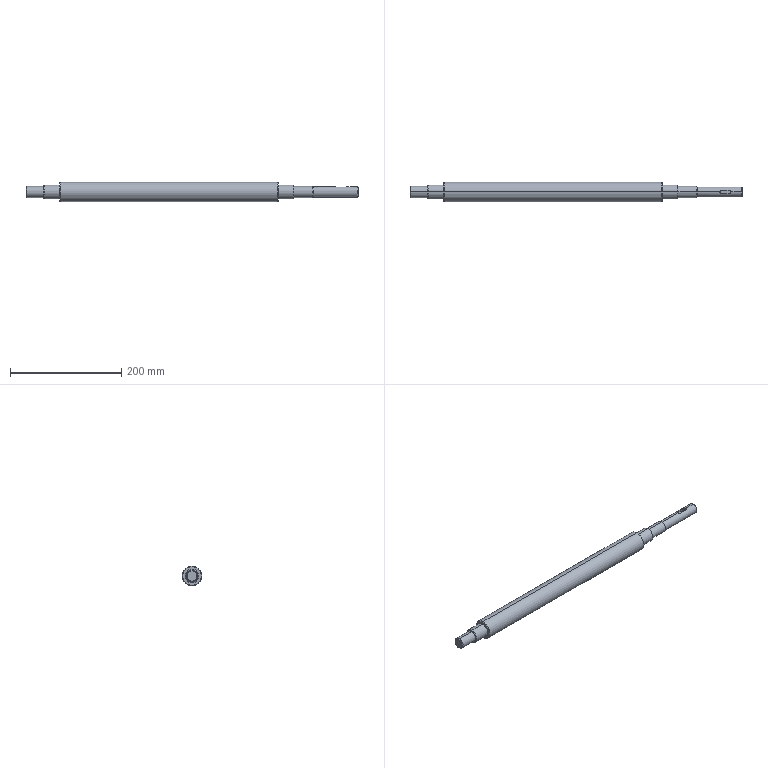Part | STEP file | Flat conveyor mechanism-CN2500x400-107-101 | 1 solid | 49 faces | box 595.6 x 35 x 35 mm | volume 445688 mm3 | cylinder 20 | cone 14 | plane 11 | torus 4 | commonest cylinder face diameters 0.4 x4 6 x4 20 x4 25 x4 18 x2 35 x2
STEP:
#1=CARTESIAN_POINT('',(-256.4,0.,9.));
#2=VERTEX_POINT('',#1);
#3=CARTESIAN_POINT('',(-256.4,0.,-9.));
#4=VERTEX_POINT('',#3);
#5=CARTESIAN_POINT('',(-256.4,0.,0.));
#6=DIRECTION('',(-1.,0.,0.));
#7=DIRECTION('',(0.,0.,-1.));
#8=AXIS2_PLACEMENT_3D('',#5,#6,#7);
#9=CIRCLE('',#8,9.);
#10=EDGE_CURVE('',#2,#4,#9,.T.);
#11=ORIENTED_EDGE('',*,*,#10,.F.);
#12=CARTESIAN_POINT('',(-255.4,0.,10.));
#13=VERTEX_POINT('',#12);
#14=CARTESIAN_POINT('',(-256.4,0.,9.));
#15=DIRECTION('',(0.7071,0.,0.7071));
#16=VECTOR('',#15,1000.);
#17=LINE('',#14,#16);
#18=EDGE_CURVE('',#2,#13,#17,.T.);
#19=ORIENTED_EDGE('',*,*,#18,.T.);
#20=CARTESIAN_POINT('',(-255.4,0.,-10.));
#21=VERTEX_POINT('',#20);
#22=CARTESIAN_POINT('',(-255.4,0.,0.));
#23=DIRECTION('',(1.,0.,0.));
#24=DIRECTION('',(0.,0.,-1.));
#25=AXIS2_PLACEMENT_3D('',#22,#23,#24);
#26=CIRCLE('',#25,10.);
#27=EDGE_CURVE('',#21,#13,#26,.T.);
#28=ORIENTED_EDGE('',*,*,#27,.F.);
#29=CARTESIAN_POINT('',(-256.4,0.,-9.));
#30=DIRECTION('',(0.7071,0.,-0.7071));
#31=VECTOR('',#30,1000.);
#32=LINE('',#29,#31);
#33=EDGE_CURVE('',#4,#21,#32,.T.);
#34=ORIENTED_EDGE('',*,*,#33,.F.);
#35=EDGE_LOOP('',(#11,#19,#28,#34));
#36=FACE_OUTER_BOUND('',#35,.T.);
#37=CARTESIAN_POINT('',(-256.4,0.,0.));
#38=DIRECTION('',(1.,0.,0.));
#39=DIRECTION('',(0.,0.,-1.));
#40=AXIS2_PLACEMENT_3D('',#37,#38,#39);
#41=CONICAL_SURFACE('',#40,9.,0.7854);
#42=ADVANCED_FACE('',(#36),#41,.T.);
#43=CARTESIAN_POINT('',(-224.4,0.,11.5));
#44=VERTEX_POINT('',#43);
#45=CARTESIAN_POINT('',(-224.4,0.,-11.5));
#46=VERTEX_POINT('',#45);
#47=CARTESIAN_POINT('',(-224.4,0.,0.));
#48=DIRECTION('',(-1.,0.,0.));
#49=DIRECTION('',(0.,0.,-1.));
#50=AXIS2_PLACEMENT_3D('',#47,#48,#49);
#51=CIRCLE('',#50,11.5);
#52=EDGE_CURVE('',#44,#46,#51,.T.);
#53=ORIENTED_EDGE('',*,*,#52,.F.);
#54=CARTESIAN_POINT('',(-223.4,0.,12.5));
#55=VERTEX_POINT('',#54);
#56=CARTESIAN_POINT('',(-224.4,0.,11.5));
#57=DIRECTION('',(0.7071,0.,0.7071));
#58=VECTOR('',#57,1000.);
#59=LINE('',#56,#58);
#60=EDGE_CURVE('',#44,#55,#59,.T.);
#61=ORIENTED_EDGE('',*,*,#60,.T.);
#62=CARTESIAN_POINT('',(-223.4,0.,-12.5));
#63=VERTEX_POINT('',#62);
#64=CARTESIAN_POINT('',(-223.4,0.,0.));
#65=DIRECTION('',(1.,0.,0.));
#66=DIRECTION('',(0.,0.,-1.));
#67=AXIS2_PLACEMENT_3D('',#64,#65,#66);
#68=CIRCLE('',#67,12.5);
#69=EDGE_CURVE('',#63,#55,#68,.T.);
#70=ORIENTED_EDGE('',*,*,#69,.F.);
#71=CARTESIAN_POINT('',(-224.4,0.,-11.5));
#72=DIRECTION('',(0.7071,0.,-0.7071));
#73=VECTOR('',#72,1000.);
#74=LINE('',#71,#73);
#75=EDGE_CURVE('',#46,#63,#74,.T.);
#76=ORIENTED_EDGE('',*,*,#75,.F.);
#77=EDGE_LOOP('',(#53,#61,#70,#76));
#78=FACE_OUTER_BOUND('',#77,.T.);
#79=CARTESIAN_POINT('',(-224.4,0.,0.));
#80=DIRECTION('',(1.,0.,0.));
#81=DIRECTION('',(0.,0.,-1.));
#82=AXIS2_PLACEMENT_3D('',#79,#80,#81);
#83=CONICAL_SURFACE('',#82,11.5,0.7854);
#84=ADVANCED_FACE('',(#78),#83,.T.);
#85=CARTESIAN_POINT('',(-196.1,0.,16.5));
#86=VERTEX_POINT('',#85);
#87=CARTESIAN_POINT('',(-196.1,0.,-16.5));
#88=VERTEX_POINT('',#87);
#89=CARTESIAN_POINT('',(-196.1,0.,0.));
#90=DIRECTION('',(-1.,0.,0.));
#91=DIRECTION('',(0.,0.,-1.));
#92=AXIS2_PLACEMENT_3D('',#89,#90,#91);
#93=CIRCLE('',#92,16.5);
#94=EDGE_CURVE('',#86,#88,#93,.T.);
#95=ORIENTED_EDGE('',*,*,#94,.F.);
#96=CARTESIAN_POINT('',(-195.1,0.,17.5));
#97=VERTEX_POINT('',#96);
#98=CARTESIAN_POINT('',(-196.1,0.,16.5));
#99=DIRECTION('',(0.7071,0.,0.7071));
#100=VECTOR('',#99,1000.);
#101=LINE('',#98,#100);
#102=EDGE_CURVE('',#86,#97,#101,.T.);
#103=ORIENTED_EDGE('',*,*,#102,.T.);
#104=CARTESIAN_POINT('',(-195.1,0.,-17.5));
#105=VERTEX_POINT('',#104);
#106=CARTESIAN_POINT('',(-195.1,0.,0.));
#107=DIRECTION('',(1.,0.,0.));
#108=DIRECTION('',(0.,0.,-1.));
#109=AXIS2_PLACEMENT_3D('',#106,#107,#108);
#110=CIRCLE('',#109,17.5);
#111=EDGE_CURVE('',#105,#97,#110,.T.);
#112=ORIENTED_EDGE('',*,*,#111,.F.);
#113=CARTESIAN_POINT('',(-196.1,0.,-16.5));
#114=DIRECTION('',(0.7071,0.,-0.7071));
#115=VECTOR('',#114,1000.);
#116=LINE('',#113,#115);
#117=EDGE_CURVE('',#88,#105,#116,.T.);
#118=ORIENTED_EDGE('',*,*,#117,.F.);
#119=EDGE_LOOP('',(#95,#103,#112,#118));
#120=FACE_OUTER_BOUND('',#119,.T.);
#121=CARTESIAN_POINT('',(-196.1,0.,0.));
#122=DIRECTION('',(1.,0.,0.));
#123=DIRECTION('',(0.,0.,-1.));
#124=AXIS2_PLACEMENT_3D('',#121,#122,#123);
#125=CONICAL_SURFACE('',#124,16.5,0.7854);
#126=ADVANCED_FACE('',(#120),#125,.T.);
#127=CARTESIAN_POINT('',(195.9,0.,-16.5));
#128=VERTEX_POINT('',#127);
#129=CARTESIAN_POINT('',(195.9,0.,16.5));
#130=VERTEX_POINT('',#129);
#131=CARTESIAN_POINT('',(195.9,0.,0.));
#132=DIRECTION('',(1.,0.,0.));
#133=DIRECTION('',(0.,0.,1.));
#134=AXIS2_PLACEMENT_3D('',#131,#132,#133);
#135=CIRCLE('',#134,16.5);
#136=EDGE_CURVE('',#128,#130,#135,.T.);
#137=ORIENTED_EDGE('',*,*,#136,.F.);
#138=CARTESIAN_POINT('',(194.9,0.,-17.5));
#139=VERTEX_POINT('',#138);
#140=CARTESIAN_POINT('',(194.9,0.,-17.5));
#141=DIRECTION('',(-0.7071,0.,-0.7071));
#142=VECTOR('',#141,1000.);
#143=LINE('',#140,#142);
#144=EDGE_CURVE('',#128,#139,#143,.T.);
#145=ORIENTED_EDGE('',*,*,#144,.T.);
#146=CARTESIAN_POINT('',(194.9,0.,17.5));
#147=VERTEX_POINT('',#146);
#148=CARTESIAN_POINT('',(194.9,0.,0.));
#149=DIRECTION('',(-1.,0.,0.));
#150=DIRECTION('',(0.,0.,1.));
#151=AXIS2_PLACEMENT_3D('',#148,#149,#150);
#152=CIRCLE('',#151,17.5);
#153=EDGE_CURVE('',#147,#139,#152,.T.);
#154=ORIENTED_EDGE('',*,*,#153,.F.);
#155=CARTESIAN_POINT('',(194.9,0.,17.5));
#156=DIRECTION('',(-0.7071,0.,0.7071));
#157=VECTOR('',#156,1000.);
#158=LINE('',#155,#157);
#159=EDGE_CURVE('',#130,#147,#158,.T.);
#160=ORIENTED_EDGE('',*,*,#159,.F.);
#161=EDGE_LOOP('',(#137,#145,#154,#160));
#162=FACE_OUTER_BOUND('',#161,.T.);
#163=CARTESIAN_POINT('',(194.9,0.,0.));
#164=DIRECTION('',(-1.,0.,0.));
#165=DIRECTION('',(0.,0.,1.));
#166=AXIS2_PLACEMENT_3D('',#163,#164,#165);
#167=CONICAL_SURFACE('',#166,17.5,0.7854);
#168=ADVANCED_FACE('',(#162),#167,.T.);
#169=CARTESIAN_POINT('',(224.2,0.,-11.5));
#170=VERTEX_POINT('',#169);
#171=CARTESIAN_POINT('',(224.2,0.,11.5));
#172=VERTEX_POINT('',#171);
#173=CARTESIAN_POINT('',(224.2,0.,0.));
#174=DIRECTION('',(1.,0.,0.));
#175=DIRECTION('',(0.,0.,1.));
#176=AXIS2_PLACEMENT_3D('',#173,#174,#175);
#177=CIRCLE('',#176,11.5);
#178=EDGE_CURVE('',#170,#172,#177,.T.);
#179=ORIENTED_EDGE('',*,*,#178,.F.);
#180=CARTESIAN_POINT('',(223.2,0.,-12.5));
#181=VERTEX_POINT('',#180);
#182=CARTESIAN_POINT('',(223.2,0.,-12.5));
#183=DIRECTION('',(-0.7071,0.,-0.7071));
#184=VECTOR('',#183,1000.);
#185=LINE('',#182,#184);
#186=EDGE_CURVE('',#170,#181,#185,.T.);
#187=ORIENTED_EDGE('',*,*,#186,.T.);
#188=CARTESIAN_POINT('',(223.2,0.,12.5));
#189=VERTEX_POINT('',#188);
#190=CARTESIAN_POINT('',(223.2,0.,0.));
#191=DIRECTION('',(-1.,0.,0.));
#192=DIRECTION('',(0.,0.,1.));
#193=AXIS2_PLACEMENT_3D('',#190,#191,#192);
#194=CIRCLE('',#193,12.5);
#195=EDGE_CURVE('',#189,#181,#194,.T.);
#196=ORIENTED_EDGE('',*,*,#195,.F.);
#197=CARTESIAN_POINT('',(223.2,0.,12.5));
#198=DIRECTION('',(-0.7071,0.,0.7071));
#199=VECTOR('',#198,1000.);
#200=LINE('',#197,#199);
#201=EDGE_CURVE('',#172,#189,#200,.T.);
#202=ORIENTED_EDGE('',*,*,#201,.F.);
#203=EDGE_LOOP('',(#179,#187,#196,#202));
#204=FACE_OUTER_BOUND('',#203,.T.);
#205=CARTESIAN_POINT('',(223.2,0.,0.));
#206=DIRECTION('',(-1.,0.,0.));
#207=DIRECTION('',(0.,0.,1.));
#208=AXIS2_PLACEMENT_3D('',#205,#206,#207);
#209=CONICAL_SURFACE('',#208,12.5,0.7854);
#210=ADVANCED_FACE('',(#204),#209,.T.);
#211=CARTESIAN_POINT('',(259.2,0.,9.));
#212=VERTEX_POINT('',#211);
#213=CARTESIAN_POINT('',(259.2,0.,-9.));
#214=VERTEX_POINT('',#213);
#215=CARTESIAN_POINT('',(259.2,0.,0.));
#216=DIRECTION('',(-1.,0.,0.));
#217=DIRECTION('',(0.,0.,1.));
#218=AXIS2_PLACEMENT_3D('',#215,#216,#217);
#219=CIRCLE('',#218,9.);
#220=EDGE_CURVE('',#212,#214,#219,.T.);
#221=ORIENTED_EDGE('',*,*,#220,.T.);
#222=CARTESIAN_POINT('',(258.2,0.,-10.));
#223=VERTEX_POINT('',#222);
#224=CARTESIAN_POINT('',(258.2,0.,-10.));
#225=DIRECTION('',(-0.7071,0.,-0.7071));
#226=VECTOR('',#225,1000.);
#227=LINE('',#224,#226);
#228=EDGE_CURVE('',#214,#223,#227,.T.);
#229=ORIENTED_EDGE('',*,*,#228,.T.);
#230=CARTESIAN_POINT('',(258.2,0.,10.));
#231=VERTEX_POINT('',#230);
#232=CARTESIAN_POINT('',(258.2,0.,0.));
#233=DIRECTION('',(-1.,0.,0.));
#234=DIRECTION('',(0.,0.,1.));
#235=AXIS2_PLACEMENT_3D('',#232,#233,#234);
#236=CIRCLE('',#235,10.);
#237=EDGE_CURVE('',#231,#223,#236,.T.);
#238=ORIENTED_EDGE('',*,*,#237,.F.);
#239=CARTESIAN_POINT('',(258.2,0.,10.));
#240=DIRECTION('',(-0.7071,0.,0.7071));
#241=VECTOR('',#240,1000.);
#242=LINE('',#239,#241);
#243=EDGE_CURVE('',#212,#231,#242,.T.);
#244=ORIENTED_EDGE('',*,*,#243,.F.);
#245=EDGE_LOOP('',(#221,#229,#238,#244));
#246=FACE_OUTER_BOUND('',#245,.T.);
#247=CARTESIAN_POINT('',(258.2,0.,0.));
#248=DIRECTION('',(-1.,0.,0.));
#249=DIRECTION('',(0.,0.,1.));
#250=AXIS2_PLACEMENT_3D('',#247,#248,#249);
#251=CONICAL_SURFACE('',#250,10.,0.7854);
#252=ADVANCED_FACE('',(#246),#251,.T.);
#253=CARTESIAN_POINT('',(339.2,0.,-8.));
#254=VERTEX_POINT('',#253);
#255=CARTESIAN_POINT('',(339.2,0.,8.));
#256=VERTEX_POINT('',#255);
#257=CARTESIAN_POINT('',(339.2,0.,0.));
#258=DIRECTION('',(1.,0.,0.));
#259=DIRECTION('',(0.,0.,1.));
#260=AXIS2_PLACEMENT_3D('',#257,#258,#259);
#261=CIRCLE('',#260,8.);
#262=EDGE_CURVE('',#254,#256,#261,.T.);
#263=ORIENTED_EDGE('',*,*,#262,.F.);
#264=CARTESIAN_POINT('',(338.2,0.,-9.));
#265=VERTEX_POINT('',#264);
#266=CARTESIAN_POINT('',(338.2,0.,-9.));
#267=DIRECTION('',(-0.7071,0.,-0.7071));
#268=VECTOR('',#267,1000.);
#269=LINE('',#266,#268);
#270=EDGE_CURVE('',#254,#265,#269,.T.);
#271=ORIENTED_EDGE('',*,*,#270,.T.);
#272=CARTESIAN_POINT('',(338.2,0.,9.));
#273=VERTEX_POINT('',#272);
#274=CARTESIAN_POINT('',(338.2,0.,0.));
#275=DIRECTION('',(-1.,0.,0.));
#276=DIRECTION('',(0.,0.,1.));
#277=AXIS2_PLACEMENT_3D('',#274,#275,#276);
#278=CIRCLE('',#277,9.);
#279=EDGE_CURVE('',#273,#265,#278,.T.);
#280=ORIENTED_EDGE('',*,*,#279,.F.);
#281=CARTESIAN_POINT('',(338.2,0.,9.));
#282=DIRECTION('',(-0.7071,0.,0.7071));
#283=VECTOR('',#282,1000.);
#284=LINE('',#281,#283);
#285=EDGE_CURVE('',#256,#273,#284,.T.);
#286=ORIENTED_EDGE('',*,*,#285,.F.);
#287=EDGE_LOOP('',(#263,#271,#280,#286));
#288=FACE_OUTER_BOUND('',#287,.T.);
#289=CARTESIAN_POINT('',(338.2,0.,0.));
#290=DIRECTION('',(-1.,0.,0.));
#291=DIRECTION('',(0.,0.,1.));
#292=AXIS2_PLACEMENT_3D('',#289,#290,#291);
#293=CONICAL_SURFACE('',#292,9.,0.7854);
#294=ADVANCED_FACE('',(#288),#293,.T.);
#295=CARTESIAN_POINT('',(-224.4,0.,10.));
#296=VERTEX_POINT('',#295);
#297=CARTESIAN_POINT('',(-224.4,0.,-10.));
#298=VERTEX_POINT('',#297);
#299=CARTESIAN_POINT('',(-224.4,0.,0.));
#300=DIRECTION('',(-1.,0.,0.));
#301=DIRECTION('',(0.,0.,1.));
#302=AXIS2_PLACEMENT_3D('',#299,#300,#301);
#303=CIRCLE('',#302,10.);
#304=EDGE_CURVE('',#296,#298,#303,.T.);
#305=ORIENTED_EDGE('',*,*,#304,.T.);
#306=CARTESIAN_POINT('',(-209.5,0.,-10.));
#307=DIRECTION('',(-1.,0.,0.));
#308=VECTOR('',#307,1000.);
#309=LINE('',#306,#308);
#310=EDGE_CURVE('',#298,#21,#309,.T.);
#311=ORIENTED_EDGE('',*,*,#310,.T.);
#312=ORIENTED_EDGE('',*,*,#27,.T.);
#313=CARTESIAN_POINT('',(-209.5,0.,10.));
#314=DIRECTION('',(-1.,0.,0.));
#315=VECTOR('',#314,1000.);
#316=LINE('',#313,#315);
#317=EDGE_CURVE('',#296,#13,#316,.T.);
#318=ORIENTED_EDGE('',*,*,#317,.F.);
#319=EDGE_LOOP('',(#305,#311,#312,#318));
#320=FACE_OUTER_BOUND('',#319,.T.);
#321=CARTESIAN_POINT('',(-209.5,0.,0.));
#322=DIRECTION('',(-1.,0.,0.));
#323=DIRECTION('',(0.,0.,1.));
#324=AXIS2_PLACEMENT_3D('',#321,#322,#323);
#325=CYLINDRICAL_SURFACE('',#324,10.);
#326=ADVANCED_FACE('',(#320),#325,.T.);
#327=CARTESIAN_POINT('',(-196.1,0.,12.5));
#328=VERTEX_POINT('',#327);
#329=CARTESIAN_POINT('',(-196.1,0.,-12.5));
#330=VERTEX_POINT('',#329);
#331=CARTESIAN_POINT('',(-196.1,0.,0.));
#332=DIRECTION('',(-1.,0.,0.));
#333=DIRECTION('',(0.,0.,1.));
#334=AXIS2_PLACEMENT_3D('',#331,#332,#333);
#335=CIRCLE('',#334,12.5);
#336=EDGE_CURVE('',#328,#330,#335,.T.);
#337=ORIENTED_EDGE('',*,*,#336,.T.);
#338=CARTESIAN_POINT('',(-209.5,0.,-12.5));
#339=DIRECTION('',(-1.,0.,0.));
#340=VECTOR('',#339,1000.);
#341=LINE('',#338,#340);
#342=EDGE_CURVE('',#330,#63,#341,.T.);
#343=ORIENTED_EDGE('',*,*,#342,.T.);
#344=ORIENTED_EDGE('',*,*,#69,.T.);
#345=CARTESIAN_POINT('',(-209.5,0.,12.5));
#346=DIRECTION('',(-1.,0.,0.));
#347=VECTOR('',#346,1000.);
#348=LINE('',#345,#347);
#349=EDGE_CURVE('',#328,#55,#348,.T.);
#350=ORIENTED_EDGE('',*,*,#349,.F.);
#351=EDGE_LOOP('',(#337,#343,#344,#350));
#352=FACE_OUTER_BOUND('',#351,.T.);
#353=CARTESIAN_POINT('',(-209.5,0.,0.));
#354=DIRECTION('',(-1.,0.,0.));
#355=DIRECTION('',(0.,0.,1.));
#356=AXIS2_PLACEMENT_3D('',#353,#354,#355);
#357=CYLINDRICAL_SURFACE('',#356,12.5);
#358=ADVANCED_FACE('',(#352),#357,.T.);
#359=ORIENTED_EDGE('',*,*,#153,.T.);
#360=CARTESIAN_POINT('',(-209.5,0.,-17.5));
#361=DIRECTION('',(-1.,0.,0.));
#362=VECTOR('',#361,1000.);
#363=LINE('',#360,#362);
#364=EDGE_CURVE('',#139,#105,#363,.T.);
#365=ORIENTED_EDGE('',*,*,#364,.T.);
#366=ORIENTED_EDGE('',*,*,#111,.T.);
#367=CARTESIAN_POINT('',(-209.5,0.,17.5));
#368=DIRECTION('',(-1.,0.,0.));
#369=VECTOR('',#368,1000.);
#370=LINE('',#367,#369);
#371=EDGE_CURVE('',#147,#97,#370,.T.);
#372=ORIENTED_EDGE('',*,*,#371,.F.);
#373=EDGE_LOOP('',(#359,#365,#366,#372));
#374=FACE_OUTER_BOUND('',#373,.T.);
#375=CARTESIAN_POINT('',(-209.5,0.,0.));
#376=DIRECTION('',(-1.,0.,0.));
#377=DIRECTION('',(0.,0.,1.));
#378=AXIS2_PLACEMENT_3D('',#375,#376,#377);
#379=CYLINDRICAL_SURFACE('',#378,17.5);
#380=ADVANCED_FACE('',(#374),#379,.T.);
#381=ORIENTED_EDGE('',*,*,#195,.T.);
#382=CARTESIAN_POINT('',(195.9,0.,-12.5));
#383=VERTEX_POINT('',#382);
#384=CARTESIAN_POINT('',(-209.5,0.,-12.5));
#385=DIRECTION('',(-1.,0.,0.));
#386=VECTOR('',#385,1000.);
#387=LINE('',#384,#386);
#388=EDGE_CURVE('',#181,#383,#387,.T.);
#389=ORIENTED_EDGE('',*,*,#388,.T.);
#390=CARTESIAN_POINT('',(195.9,0.,12.5));
#391=VERTEX_POINT('',#390);
#392=CARTESIAN_POINT('',(195.9,0.,0.));
#393=DIRECTION('',(-1.,0.,0.));
#394=DIRECTION('',(0.,0.,1.));
#395=AXIS2_PLACEMENT_3D('',#392,#393,#394);
#396=CIRCLE('',#395,12.5);
#397=EDGE_CURVE('',#391,#383,#396,.T.);
#398=ORIENTED_EDGE('',*,*,#397,.F.);
#399=CARTESIAN_POINT('',(-209.5,0.,12.5));
#400=DIRECTION('',(-1.,0.,0.));
#401=VECTOR('',#400,1000.);
#402=LINE('',#399,#401);
#403=EDGE_CURVE('',#189,#391,#402,.T.);
#404=ORIENTED_EDGE('',*,*,#403,.F.);
#405=EDGE_LOOP('',(#381,#389,#398,#404));
#406=FACE_OUTER_BOUND('',#405,.T.);
#407=CARTESIAN_POINT('',(-209.5,0.,0.));
#408=DIRECTION('',(-1.,0.,0.));
#409=DIRECTION('',(0.,0.,1.));
#410=AXIS2_PLACEMENT_3D('',#407,#408,#409);
#411=CYLINDRICAL_SURFACE('',#410,12.5);
#412=ADVANCED_FACE('',(#406),#411,.T.);
#413=ORIENTED_EDGE('',*,*,#237,.T.);
#414=CARTESIAN_POINT('',(224.2,0.,-10.));
#415=VERTEX_POINT('',#414);
#416=CARTESIAN_POINT('',(-209.5,0.,-10.));
#417=DIRECTION('',(-1.,0.,0.));
#418=VECTOR('',#417,1000.);
#419=LINE('',#416,#418);
#420=EDGE_CURVE('',#223,#415,#419,.T.);
#421=ORIENTED_EDGE('',*,*,#420,.T.);
#422=CARTESIAN_POINT('',(224.2,0.,10.));
#423=VERTEX_POINT('',#422);
#424=CARTESIAN_POINT('',(224.2,0.,0.));
#425=DIRECTION('',(-1.,0.,0.));
#426=DIRECTION('',(0.,0.,1.));
#427=AXIS2_PLACEMENT_3D('',#424,#425,#426);
#428=CIRCLE('',#427,10.);
#429=EDGE_CURVE('',#423,#415,#428,.T.);
#430=ORIENTED_EDGE('',*,*,#429,.F.);
#431=CARTESIAN_POINT('',(-209.5,0.,10.));
#432=DIRECTION('',(-1.,0.,0.));
#433=VECTOR('',#432,1000.);
#434=LINE('',#431,#433);
#435=EDGE_CURVE('',#231,#423,#434,.T.);
#436=ORIENTED_EDGE('',*,*,#435,.F.);
#437=EDGE_LOOP('',(#413,#421,#430,#436));
#438=FACE_OUTER_BOUND('',#437,.T.);
#439=CARTESIAN_POINT('',(-209.5,0.,0.));
#440=DIRECTION('',(-1.,0.,0.));
#441=DIRECTION('',(0.,0.,1.));
#442=AXIS2_PLACEMENT_3D('',#439,#440,#441);
#443=CYLINDRICAL_SURFACE('',#442,10.);
#444=ADVANCED_FACE('',(#438),#443,.T.);
#445=ORIENTED_EDGE('',*,*,#279,.T.);
#446=CARTESIAN_POINT('',(-209.5,0.,-9.));
#447=DIRECTION('',(-1.,0.,0.));
#448=VECTOR('',#447,1000.);
#449=LINE('',#446,#448);
#450=EDGE_CURVE('',#265,#214,#449,.T.);
#451=ORIENTED_EDGE('',*,*,#450,.T.);
#452=ORIENTED_EDGE('',*,*,#220,.F.);
#453=CARTESIAN_POINT('',(299.2,0.,9.));
#454=VERTEX_POINT('',#453);
#455=CARTESIAN_POINT('',(-209.5,0.,9.));
#456=DIRECTION('',(-1.,0.,0.));
#457=VECTOR('',#456,1000.);
#458=LINE('',#455,#457);
#459=EDGE_CURVE('',#454,#212,#458,.T.);
#460=ORIENTED_EDGE('',*,*,#459,.F.);
#461=CARTESIAN_POINT('',(302.2,3.,8.485));
#462=VERTEX_POINT('',#461);
#463=CARTESIAN_POINT('',(299.2,0.,9.));
#464=CARTESIAN_POINT('',(299.2,0.1996,9.));
#465=CARTESIAN_POINT('',(299.22,0.3957,8.993));
#466=CARTESIAN_POINT('',(299.297,0.7809,8.968));
#467=CARTESIAN_POINT('',(299.355,0.9721,8.949));
#468=CARTESIAN_POINT('',(299.506,1.335,8.902));
#469=CARTESIAN_POINT('',(299.598,1.506,8.875));
#470=CARTESIAN_POINT('',(299.816,1.831,8.813));
#471=CARTESIAN_POINT('',(299.941,1.984,8.78));
#472=CARTESIAN_POINT('',(300.353,2.396,8.68));
#473=CARTESIAN_POINT('',(300.685,2.618,8.612));
#474=CARTESIAN_POINT('',(301.225,2.844,8.539));
#475=CARTESIAN_POINT('',(301.415,2.902,8.519));
#476=CARTESIAN_POINT('',(301.803,2.98,8.492));
#477=CARTESIAN_POINT('',(302.,3.,8.485));
#478=CARTESIAN_POINT('',(302.2,3.,8.485));
#479=B_SPLINE_CURVE_WITH_KNOTS('',3,(#463,#464,#465,#466,#467,#468,#469,#470,#471,#472,#473,#474,#475,#476,#477,#478),.UNSPECIFIED.,.F.,.F.,(4,2,2,2,2,2,2,4),(0.,0.0005901,0.00118,0.00177,0.00236,0.003541,0.004131,0.004721),.UNSPECIFIED.);
#480=EDGE_CURVE('',#454,#462,#479,.T.);
#481=ORIENTED_EDGE('',*,*,#480,.T.);
#482=CARTESIAN_POINT('',(316.2,3.,8.485));
#483=VERTEX_POINT('',#482);
#484=CARTESIAN_POINT('',(-209.5,3.,8.485));
#485=DIRECTION('',(1.,0.,0.));
#486=VECTOR('',#485,1000.);
#487=LINE('',#484,#486);
#488=EDGE_CURVE('',#462,#483,#487,.T.);
#489=ORIENTED_EDGE('',*,*,#488,.T.);
#490=CARTESIAN_POINT('',(319.2,0.,9.));
#491=VERTEX_POINT('',#490);
#492=CARTESIAN_POINT('',(316.2,3.,8.485));
#493=CARTESIAN_POINT('',(316.4,3.,8.485));
#494=CARTESIAN_POINT('',(316.596,2.98,8.492));
#495=CARTESIAN_POINT('',(316.981,2.903,8.519));
#496=CARTESIAN_POINT('',(317.172,2.845,8.539));
#497=CARTESIAN_POINT('',(317.534,2.694,8.588));
#498=CARTESIAN_POINT('',(317.706,2.602,8.616));
#499=CARTESIAN_POINT('',(318.031,2.385,8.679));
#500=CARTESIAN_POINT('',(318.183,2.259,8.713));
#501=CARTESIAN_POINT('',(318.595,1.848,8.813));
#502=CARTESIAN_POINT('',(318.818,1.516,8.879));
#503=CARTESIAN_POINT('',(319.044,0.9753,8.949));
#504=CARTESIAN_POINT('',(319.102,0.7852,8.968));
#505=CARTESIAN_POINT('',(319.18,0.3966,8.993));
#506=CARTESIAN_POINT('',(319.2,0.1996,9.));
#507=CARTESIAN_POINT('',(319.2,0.,9.));
#508=B_SPLINE_CURVE_WITH_KNOTS('',3,(#492,#493,#494,#495,#496,#497,#498,#499,#500,#501,#502,#503,#504,#505,#506,#507),.UNSPECIFIED.,.F.,.F.,(4,2,2,2,2,2,2,4),(0.,0.0005901,0.00118,0.00177,0.00236,0.00354,0.00413,0.004721),.UNSPECIFIED.);
#509=EDGE_CURVE('',#483,#491,#508,.T.);
#510=ORIENTED_EDGE('',*,*,#509,.T.);
#511=CARTESIAN_POINT('',(-209.5,0.,9.));
#512=DIRECTION('',(-1.,0.,0.));
#513=VECTOR('',#512,1000.);
#514=LINE('',#511,#513);
#515=EDGE_CURVE('',#273,#491,#514,.T.);
#516=ORIENTED_EDGE('',*,*,#515,.F.);
#517=EDGE_LOOP('',(#445,#451,#452,#460,#481,#489,#510,#516));
#518=FACE_OUTER_BOUND('',#517,.T.);
#519=CARTESIAN_POINT('',(-209.5,0.,0.));
#520=DIRECTION('',(-1.,0.,0.));
#521=DIRECTION('',(0.,0.,1.));
#522=AXIS2_PLACEMENT_3D('',#519,#520,#521);
#523=CYLINDRICAL_SURFACE('',#522,9.);
#524=ADVANCED_FACE('',(#518),#523,.T.);
#525=CARTESIAN_POINT('',(-256.4,0.,0.));
#526=DIRECTION('',(-1.,0.,0.));
#527=DIRECTION('',(0.,0.,-1.));
#528=AXIS2_PLACEMENT_3D('',#525,#526,#527);
#529=CIRCLE('',#528,9.);
#530=EDGE_CURVE('',#4,#2,#529,.T.);
#531=ORIENTED_EDGE('',*,*,#530,.T.);
#532=ORIENTED_EDGE('',*,*,#10,.T.);
#533=EDGE_LOOP('',(#531,#532));
#534=FACE_OUTER_BOUND('',#533,.T.);
#535=CARTESIAN_POINT('',(-256.4,0.,-10.));
#536=DIRECTION('',(1.,0.,0.));
#537=DIRECTION('',(0.,0.,-1.));
#538=AXIS2_PLACEMENT_3D('',#535,#536,#537);
#539=PLANE('',#538);
#540=ADVANCED_FACE('',(#534),#539,.F.);
#541=CARTESIAN_POINT('',(339.2,0.,0.));
#542=DIRECTION('',(1.,0.,0.));
#543=DIRECTION('',(0.,0.,1.));
#544=AXIS2_PLACEMENT_3D('',#541,#542,#543);
#545=CIRCLE('',#544,8.);
#546=EDGE_CURVE('',#256,#254,#545,.T.);
#547=ORIENTED_EDGE('',*,*,#546,.T.);
#548=ORIENTED_EDGE('',*,*,#262,.T.);
#549=EDGE_LOOP('',(#547,#548));
#550=FACE_OUTER_BOUND('',#549,.T.);
#551=CARTESIAN_POINT('',(339.2,0.,0.));
#552=DIRECTION('',(-1.,0.,0.));
#553=DIRECTION('',(0.,0.,1.));
#554=AXIS2_PLACEMENT_3D('',#551,#552,#553);
#555=PLANE('',#554);
#556=ADVANCED_FACE('',(#550),#555,.F.);
#557=ORIENTED_EDGE('',*,*,#450,.F.);
#558=CARTESIAN_POINT('',(338.2,0.,0.));
#559=DIRECTION('',(-1.,0.,0.));
#560=DIRECTION('',(0.,0.,1.));
#561=AXIS2_PLACEMENT_3D('',#558,#559,#560);
#562=CIRCLE('',#561,9.);
#563=EDGE_CURVE('',#265,#273,#562,.T.);
#564=ORIENTED_EDGE('',*,*,#563,.T.);
#565=ORIENTED_EDGE('',*,*,#515,.T.);
#566=CARTESIAN_POINT('',(319.2,-0.04707,9.));
#567=VERTEX_POINT('',#566);
#568=CARTESIAN_POINT('',(319.2,0.,0.));
#569=DIRECTION('',(1.,0.,0.));
#570=DIRECTION('',(0.,0.,-1.));
#571=AXIS2_PLACEMENT_3D('',#568,#569,#570);
#572=CIRCLE('',#571,9.);
#573=EDGE_CURVE('',#491,#567,#572,.T.);
#574=ORIENTED_EDGE('',*,*,#573,.T.);
#575=CARTESIAN_POINT('',(316.2,-3.047,8.468));
#576=VERTEX_POINT('',#575);
#577=CARTESIAN_POINT('',(319.2,-0.04707,9.));
#578=CARTESIAN_POINT('',(319.2,-0.2468,8.999));
#579=CARTESIAN_POINT('',(319.18,-0.4428,8.991));
#580=CARTESIAN_POINT('',(319.103,-0.8281,8.964));
#581=CARTESIAN_POINT('',(319.045,-1.019,8.944));
#582=CARTESIAN_POINT('',(318.894,-1.382,8.895));
#583=CARTESIAN_POINT('',(318.802,-1.553,8.866));
#584=CARTESIAN_POINT('',(318.584,-1.878,8.803));
#585=CARTESIAN_POINT('',(318.459,-2.031,8.769));
#586=CARTESIAN_POINT('',(318.047,-2.443,8.667));
#587=CARTESIAN_POINT('',(317.716,-2.665,8.598));
#588=CARTESIAN_POINT('',(317.175,-2.891,8.523));
#589=CARTESIAN_POINT('',(316.985,-2.949,8.503));
#590=CARTESIAN_POINT('',(316.597,-3.027,8.476));
#591=CARTESIAN_POINT('',(316.4,-3.047,8.468));
#592=CARTESIAN_POINT('',(316.2,-3.047,8.468));
#593=B_SPLINE_CURVE_WITH_KNOTS('',3,(#577,#578,#579,#580,#581,#582,#583,#584,#585,#586,#587,#588,#589,#590,#591,#592),.UNSPECIFIED.,.F.,.F.,(4,2,2,2,2,2,2,4),(0.,0.0005903,0.001181,0.001771,0.002361,0.003542,0.004132,0.004723),.UNSPECIFIED.);
#594=EDGE_CURVE('',#567,#576,#593,.T.);
#595=ORIENTED_EDGE('',*,*,#594,.T.);
#596=CARTESIAN_POINT('',(302.2,-3.047,8.468));
#597=VERTEX_POINT('',#596);
#598=CARTESIAN_POINT('',(-209.5,-3.047,8.468));
#599=DIRECTION('',(-1.,0.,0.));
#600=VECTOR('',#599,1000.);
#601=LINE('',#598,#600);
#602=EDGE_CURVE('',#576,#597,#601,.T.);
#603=ORIENTED_EDGE('',*,*,#602,.T.);
#604=CARTESIAN_POINT('',(299.2,-0.04707,9.));
#605=VERTEX_POINT('',#604);
#606=CARTESIAN_POINT('',(302.2,-3.047,8.468));
#607=CARTESIAN_POINT('',(302.,-3.047,8.468));
#608=CARTESIAN_POINT('',(301.804,-3.027,8.476));
#609=CARTESIAN_POINT('',(301.419,-2.95,8.503));
#610=CARTESIAN_POINT('',(301.228,-2.892,8.523));
#611=CARTESIAN_POINT('',(300.865,-2.741,8.573));
#612=CARTESIAN_POINT('',(300.694,-2.649,8.602));
#613=CARTESIAN_POINT('',(300.369,-2.431,8.666));
#614=CARTESIAN_POINT('',(300.216,-2.306,8.701));
#615=CARTESIAN_POINT('',(299.805,-1.895,8.803));
#616=CARTESIAN_POINT('',(299.582,-1.563,8.871));
#617=CARTESIAN_POINT('',(299.356,-1.023,8.944));
#618=CARTESIAN_POINT('',(299.298,-0.8324,8.964));
#619=CARTESIAN_POINT('',(299.22,-0.4437,8.991));
#620=CARTESIAN_POINT('',(299.2,-0.2468,8.999));
#621=CARTESIAN_POINT('',(299.2,-0.04707,9.));
#622=B_SPLINE_CURVE_WITH_KNOTS('',3,(#606,#607,#608,#609,#610,#611,#612,#613,#614,#615,#616,#617,#618,#619,#620,#621),.UNSPECIFIED.,.F.,.F.,(4,2,2,2,2,2,2,4),(0.,0.0005903,0.001181,0.001771,0.002361,0.003542,0.004132,0.004722),.UNSPECIFIED.);
#623=EDGE_CURVE('',#597,#605,#622,.T.);
#624=ORIENTED_EDGE('',*,*,#623,.T.);
#625=CARTESIAN_POINT('',(299.2,0.,0.));
#626=DIRECTION('',(-1.,0.,0.));
#627=DIRECTION('',(0.,0.,1.));
#628=AXIS2_PLACEMENT_3D('',#625,#626,#627);
#629=CIRCLE('',#628,9.);
#630=EDGE_CURVE('',#605,#454,#629,.T.);
#631=ORIENTED_EDGE('',*,*,#630,.T.);
#632=ORIENTED_EDGE('',*,*,#459,.T.);
#633=CARTESIAN_POINT('',(259.2,0.,0.));
#634=DIRECTION('',(-1.,0.,0.));
#635=DIRECTION('',(0.,0.,1.));
#636=AXIS2_PLACEMENT_3D('',#633,#634,#635);
#637=CIRCLE('',#636,9.);
#638=EDGE_CURVE('',#214,#212,#637,.T.);
#639=ORIENTED_EDGE('',*,*,#638,.F.);
#640=EDGE_LOOP('',(#557,#564,#565,#574,#595,#603,#624,#631,#632,#639));
#641=FACE_OUTER_BOUND('',#640,.T.);
#642=CARTESIAN_POINT('',(-209.5,0.,0.));
#643=DIRECTION('',(-1.,0.,0.));
#644=DIRECTION('',(0.,0.,1.));
#645=AXIS2_PLACEMENT_3D('',#642,#643,#644);
#646=CYLINDRICAL_SURFACE('',#645,9.);
#647=ADVANCED_FACE('',(#641),#646,.T.);
#648=ORIENTED_EDGE('',*,*,#420,.F.);
#649=CARTESIAN_POINT('',(258.2,0.,0.));
#650=DIRECTION('',(-1.,0.,0.));
#651=DIRECTION('',(0.,0.,1.));
#652=AXIS2_PLACEMENT_3D('',#649,#650,#651);
#653=CIRCLE('',#652,10.);
#654=EDGE_CURVE('',#223,#231,#653,.T.);
#655=ORIENTED_EDGE('',*,*,#654,.T.);
#656=ORIENTED_EDGE('',*,*,#435,.T.);
#657=CARTESIAN_POINT('',(224.2,0.,0.));
#658=DIRECTION('',(-1.,0.,0.));
#659=DIRECTION('',(0.,0.,1.));
#660=AXIS2_PLACEMENT_3D('',#657,#658,#659);
#661=CIRCLE('',#660,10.);
#662=EDGE_CURVE('',#415,#423,#661,.T.);
#663=ORIENTED_EDGE('',*,*,#662,.F.);
#664=EDGE_LOOP('',(#648,#655,#656,#663));
#665=FACE_OUTER_BOUND('',#664,.T.);
#666=CARTESIAN_POINT('',(-209.5,0.,0.));
#667=DIRECTION('',(-1.,0.,0.));
#668=DIRECTION('',(0.,0.,1.));
#669=AXIS2_PLACEMENT_3D('',#666,#667,#668);
#670=CYLINDRICAL_SURFACE('',#669,10.);
#671=ADVANCED_FACE('',(#665),#670,.T.);
#672=CARTESIAN_POINT('',(224.2,0.,0.));
#673=DIRECTION('',(1.,0.,0.));
#674=DIRECTION('',(0.,0.,1.));
#675=AXIS2_PLACEMENT_3D('',#672,#673,#674);
#676=CIRCLE('',#675,11.5);
#677=EDGE_CURVE('',#172,#170,#676,.T.);
#678=ORIENTED_EDGE('',*,*,#677,.T.);
#679=ORIENTED_EDGE('',*,*,#178,.T.);
#680=EDGE_LOOP('',(#678,#679));
#681=FACE_OUTER_BOUND('',#680,.T.);
#682=ORIENTED_EDGE('',*,*,#429,.T.);
#683=ORIENTED_EDGE('',*,*,#662,.T.);
#684=EDGE_LOOP('',(#682,#683));
#685=FACE_BOUND('',#684,.T.);
#686=CARTESIAN_POINT('',(224.2,0.,-12.5));
#687=DIRECTION('',(-1.,0.,0.));
#688=DIRECTION('',(0.,0.,1.));
#689=AXIS2_PLACEMENT_3D('',#686,#687,#688);
#690=PLANE('',#689);
#691=ADVANCED_FACE('',(#681,#685),#690,.F.);
#692=ORIENTED_EDGE('',*,*,#388,.F.);
#693=CARTESIAN_POINT('',(223.2,0.,0.));
#694=DIRECTION('',(-1.,0.,0.));
#695=DIRECTION('',(0.,0.,1.));
#696=AXIS2_PLACEMENT_3D('',#693,#694,#695);
#697=CIRCLE('',#696,12.5);
#698=EDGE_CURVE('',#181,#189,#697,.T.);
#699=ORIENTED_EDGE('',*,*,#698,.T.);
#700=ORIENTED_EDGE('',*,*,#403,.T.);
#701=CARTESIAN_POINT('',(195.9,0.,0.));
#702=DIRECTION('',(-1.,0.,0.));
#703=DIRECTION('',(0.,0.,1.));
#704=AXIS2_PLACEMENT_3D('',#701,#702,#703);
#705=CIRCLE('',#704,12.5);
#706=EDGE_CURVE('',#383,#391,#705,.T.);
#707=ORIENTED_EDGE('',*,*,#706,.F.);
#708=EDGE_LOOP('',(#692,#699,#700,#707));
#709=FACE_OUTER_BOUND('',#708,.T.);
#710=CARTESIAN_POINT('',(-209.5,0.,0.));
#711=DIRECTION('',(-1.,0.,0.));
#712=DIRECTION('',(0.,0.,1.));
#713=AXIS2_PLACEMENT_3D('',#710,#711,#712);
#714=CYLINDRICAL_SURFACE('',#713,12.5);
#715=ADVANCED_FACE('',(#709),#714,.T.);
#716=CARTESIAN_POINT('',(195.9,0.,0.));
#717=DIRECTION('',(1.,0.,0.));
#718=DIRECTION('',(0.,0.,1.));
#719=AXIS2_PLACEMENT_3D('',#716,#717,#718);
#720=CIRCLE('',#719,16.5);
#721=EDGE_CURVE('',#130,#128,#720,.T.);
#722=ORIENTED_EDGE('',*,*,#721,.T.);
#723=ORIENTED_EDGE('',*,*,#136,.T.);
#724=EDGE_LOOP('',(#722,#723));
#725=FACE_OUTER_BOUND('',#724,.T.);
#726=ORIENTED_EDGE('',*,*,#397,.T.);
#727=ORIENTED_EDGE('',*,*,#706,.T.);
#728=EDGE_LOOP('',(#726,#727));
#729=FACE_BOUND('',#728,.T.);
#730=CARTESIAN_POINT('',(195.9,0.,-12.5));
#731=DIRECTION('',(-1.,0.,0.));
#732=DIRECTION('',(0.,0.,1.));
#733=AXIS2_PLACEMENT_3D('',#730,#731,#732);
#734=PLANE('',#733);
#735=ADVANCED_FACE('',(#725,#729),#734,.F.);
#736=ORIENTED_EDGE('',*,*,#364,.F.);
#737=CARTESIAN_POINT('',(194.9,0.,0.));
#738=DIRECTION('',(-1.,0.,0.));
#739=DIRECTION('',(0.,0.,1.));
#740=AXIS2_PLACEMENT_3D('',#737,#738,#739);
#741=CIRCLE('',#740,17.5);
#742=EDGE_CURVE('',#139,#147,#741,.T.);
#743=ORIENTED_EDGE('',*,*,#742,.T.);
#744=ORIENTED_EDGE('',*,*,#371,.T.);
#745=CARTESIAN_POINT('',(-195.1,0.,0.));
#746=DIRECTION('',(1.,0.,0.));
#747=DIRECTION('',(0.,0.,-1.));
#748=AXIS2_PLACEMENT_3D('',#745,#746,#747);
#749=CIRCLE('',#748,17.5);
#750=EDGE_CURVE('',#97,#105,#749,.T.);
#751=ORIENTED_EDGE('',*,*,#750,.T.);
#752=EDGE_LOOP('',(#736,#743,#744,#751));
#753=FACE_OUTER_BOUND('',#752,.T.);
#754=CARTESIAN_POINT('',(-209.5,0.,0.));
#755=DIRECTION('',(-1.,0.,0.));
#756=DIRECTION('',(0.,0.,1.));
#757=AXIS2_PLACEMENT_3D('',#754,#755,#756);
#758=CYLINDRICAL_SURFACE('',#757,17.5);
#759=ADVANCED_FACE('',(#753),#758,.T.);
#760=CARTESIAN_POINT('',(-196.1,0.,0.));
#761=DIRECTION('',(-1.,0.,0.));
#762=DIRECTION('',(0.,0.,-1.));
#763=AXIS2_PLACEMENT_3D('',#760,#761,#762);
#764=CIRCLE('',#763,16.5);
#765=EDGE_CURVE('',#88,#86,#764,.T.);
#766=ORIENTED_EDGE('',*,*,#765,.T.);
#767=ORIENTED_EDGE('',*,*,#94,.T.);
#768=EDGE_LOOP('',(#766,#767));
#769=FACE_OUTER_BOUND('',#768,.T.);
#770=ORIENTED_EDGE('',*,*,#336,.F.);
#771=CARTESIAN_POINT('',(-196.1,0.,0.));
#772=DIRECTION('',(-1.,0.,0.));
#773=DIRECTION('',(0.,0.,1.));
#774=AXIS2_PLACEMENT_3D('',#771,#772,#773);
#775=CIRCLE('',#774,12.5);
#776=EDGE_CURVE('',#330,#328,#775,.T.);
#777=ORIENTED_EDGE('',*,*,#776,.F.);
#778=EDGE_LOOP('',(#770,#777));
#779=FACE_BOUND('',#778,.T.);
#780=CARTESIAN_POINT('',(-196.1,0.,-17.5));
#781=DIRECTION('',(1.,0.,0.));
#782=DIRECTION('',(0.,0.,-1.));
#783=AXIS2_PLACEMENT_3D('',#780,#781,#782);
#784=PLANE('',#783);
#785=ADVANCED_FACE('',(#769,#779),#784,.F.);
#786=ORIENTED_EDGE('',*,*,#342,.F.);
#787=ORIENTED_EDGE('',*,*,#776,.T.);
#788=ORIENTED_EDGE('',*,*,#349,.T.);
#789=CARTESIAN_POINT('',(-223.4,0.,0.));
#790=DIRECTION('',(1.,0.,0.));
#791=DIRECTION('',(0.,0.,-1.));
#792=AXIS2_PLACEMENT_3D('',#789,#790,#791);
#793=CIRCLE('',#792,12.5);
#794=EDGE_CURVE('',#55,#63,#793,.T.);
#795=ORIENTED_EDGE('',*,*,#794,.T.);
#796=EDGE_LOOP('',(#786,#787,#788,#795));
#797=FACE_OUTER_BOUND('',#796,.T.);
#798=CARTESIAN_POINT('',(-209.5,0.,0.));
#799=DIRECTION('',(-1.,0.,0.));
#800=DIRECTION('',(0.,0.,1.));
#801=AXIS2_PLACEMENT_3D('',#798,#799,#800);
#802=CYLINDRICAL_SURFACE('',#801,12.5);
#803=ADVANCED_FACE('',(#797),#802,.T.);
#804=CARTESIAN_POINT('',(-224.4,0.,0.));
#805=DIRECTION('',(-1.,0.,0.));
#806=DIRECTION('',(0.,0.,-1.));
#807=AXIS2_PLACEMENT_3D('',#804,#805,#806);
#808=CIRCLE('',#807,11.5);
#809=EDGE_CURVE('',#46,#44,#808,.T.);
#810=ORIENTED_EDGE('',*,*,#809,.T.);
#811=ORIENTED_EDGE('',*,*,#52,.T.);
#812=EDGE_LOOP('',(#810,#811));
#813=FACE_OUTER_BOUND('',#812,.T.);
#814=ORIENTED_EDGE('',*,*,#304,.F.);
#815=CARTESIAN_POINT('',(-224.4,0.,0.));
#816=DIRECTION('',(-1.,0.,0.));
#817=DIRECTION('',(0.,0.,1.));
#818=AXIS2_PLACEMENT_3D('',#815,#816,#817);
#819=CIRCLE('',#818,10.);
#820=EDGE_CURVE('',#298,#296,#819,.T.);
#821=ORIENTED_EDGE('',*,*,#820,.F.);
#822=EDGE_LOOP('',(#814,#821));
#823=FACE_BOUND('',#822,.T.);
#824=CARTESIAN_POINT('',(-224.4,0.,-12.5));
#825=DIRECTION('',(1.,0.,0.));
#826=DIRECTION('',(0.,0.,-1.));
#827=AXIS2_PLACEMENT_3D('',#824,#825,#826);
#828=PLANE('',#827);
#829=ADVANCED_FACE('',(#813,#823),#828,.F.);
#830=ORIENTED_EDGE('',*,*,#310,.F.);
#831=ORIENTED_EDGE('',*,*,#820,.T.);
#832=ORIENTED_EDGE('',*,*,#317,.T.);
#833=CARTESIAN_POINT('',(-255.4,0.,0.));
#834=DIRECTION('',(1.,0.,0.));
#835=DIRECTION('',(0.,0.,-1.));
#836=AXIS2_PLACEMENT_3D('',#833,#834,#835);
#837=CIRCLE('',#836,10.);
#838=EDGE_CURVE('',#13,#21,#837,.T.);
#839=ORIENTED_EDGE('',*,*,#838,.T.);
#840=EDGE_LOOP('',(#830,#831,#832,#839));
#841=FACE_OUTER_BOUND('',#840,.T.);
#842=CARTESIAN_POINT('',(-209.5,0.,0.));
#843=DIRECTION('',(-1.,0.,0.));
#844=DIRECTION('',(0.,0.,1.));
#845=AXIS2_PLACEMENT_3D('',#842,#843,#844);
#846=CYLINDRICAL_SURFACE('',#845,10.);
#847=ADVANCED_FACE('',(#841),#846,.T.);
#848=CARTESIAN_POINT('',(302.2,-3.047,5.7));
#849=VERTEX_POINT('',#848);
#850=CARTESIAN_POINT('',(302.2,-3.047,5.5));
#851=DIRECTION('',(0.,0.,1.));
#852=VECTOR('',#851,1000.);
#853=LINE('',#850,#852);
#854=EDGE_CURVE('',#849,#597,#853,.T.);
#855=ORIENTED_EDGE('',*,*,#854,.F.);
#856=CARTESIAN_POINT('',(299.2,-0.04707,5.7));
#857=VERTEX_POINT('',#856);
#858=CARTESIAN_POINT('',(302.2,-0.04707,5.7));
#859=DIRECTION('',(0.,0.,-1.));
#860=DIRECTION('',(-1.,0.,0.));
#861=AXIS2_PLACEMENT_3D('',#858,#859,#860);
#862=CIRCLE('',#861,3.);
#863=EDGE_CURVE('',#849,#857,#862,.T.);
#864=ORIENTED_EDGE('',*,*,#863,.T.);
#865=CARTESIAN_POINT('',(299.2,-0.04707,5.5));
#866=DIRECTION('',(0.,0.,1.));
#867=VECTOR('',#866,1000.);
#868=LINE('',#865,#867);
#869=EDGE_CURVE('',#857,#605,#868,.T.);
#870=ORIENTED_EDGE('',*,*,#869,.T.);
#871=ORIENTED_EDGE('',*,*,#623,.F.);
#872=EDGE_LOOP('',(#855,#864,#870,#871));
#873=FACE_OUTER_BOUND('',#872,.T.);
#874=CARTESIAN_POINT('',(302.2,-0.04707,5.5));
#875=DIRECTION('',(0.,0.,1.));
#876=DIRECTION('',(1.,0.,0.));
#877=AXIS2_PLACEMENT_3D('',#874,#875,#876);
#878=CYLINDRICAL_SURFACE('',#877,3.);
#879=ADVANCED_FACE('',(#873),#878,.F.);
#880=ORIENTED_EDGE('',*,*,#869,.F.);
#881=CARTESIAN_POINT('',(299.2,0.,5.7));
#882=VERTEX_POINT('',#881);
#883=CARTESIAN_POINT('',(299.2,0.,5.7));
#884=DIRECTION('',(0.,1.,0.));
#885=VECTOR('',#884,1000.);
#886=LINE('',#883,#885);
#887=EDGE_CURVE('',#857,#882,#886,.T.);
#888=ORIENTED_EDGE('',*,*,#887,.T.);
#889=CARTESIAN_POINT('',(299.2,0.,5.5));
#890=DIRECTION('',(0.,0.,1.));
#891=VECTOR('',#890,1000.);
#892=LINE('',#889,#891);
#893=EDGE_CURVE('',#882,#454,#892,.T.);
#894=ORIENTED_EDGE('',*,*,#893,.T.);
#895=ORIENTED_EDGE('',*,*,#630,.F.);
#896=EDGE_LOOP('',(#880,#888,#894,#895));
#897=FACE_OUTER_BOUND('',#896,.T.);
#898=CARTESIAN_POINT('',(299.2,0.,5.5));
#899=DIRECTION('',(-1.,0.,0.));
#900=DIRECTION('',(0.,0.,1.));
#901=AXIS2_PLACEMENT_3D('',#898,#899,#900);
#902=PLANE('',#901);
#903=ADVANCED_FACE('',(#897),#902,.F.);
#904=ORIENTED_EDGE('',*,*,#893,.F.);
#905=CARTESIAN_POINT('',(302.2,3.,5.7));
#906=VERTEX_POINT('',#905);
#907=CARTESIAN_POINT('',(302.2,0.,5.7));
#908=DIRECTION('',(0.,0.,-1.));
#909=DIRECTION('',(-1.,0.,0.));
#910=AXIS2_PLACEMENT_3D('',#907,#908,#909);
#911=CIRCLE('',#910,3.);
#912=EDGE_CURVE('',#882,#906,#911,.T.);
#913=ORIENTED_EDGE('',*,*,#912,.T.);
#914=CARTESIAN_POINT('',(302.2,3.,5.5));
#915=DIRECTION('',(0.,0.,1.));
#916=VECTOR('',#915,1000.);
#917=LINE('',#914,#916);
#918=EDGE_CURVE('',#906,#462,#917,.T.);
#919=ORIENTED_EDGE('',*,*,#918,.T.);
#920=ORIENTED_EDGE('',*,*,#480,.F.);
#921=EDGE_LOOP('',(#904,#913,#919,#920));
#922=FACE_OUTER_BOUND('',#921,.T.);
#923=CARTESIAN_POINT('',(302.2,0.,5.5));
#924=DIRECTION('',(0.,0.,1.));
#925=DIRECTION('',(1.,0.,0.));
#926=AXIS2_PLACEMENT_3D('',#923,#924,#925);
#927=CYLINDRICAL_SURFACE('',#926,3.);
#928=ADVANCED_FACE('',(#922),#927,.F.);
#929=ORIENTED_EDGE('',*,*,#918,.F.);
#930=CARTESIAN_POINT('',(316.2,3.,5.7));
#931=VERTEX_POINT('',#930);
#932=CARTESIAN_POINT('',(316.2,3.,5.7));
#933=DIRECTION('',(1.,0.,0.));
#934=VECTOR('',#933,1000.);
#935=LINE('',#932,#934);
#936=EDGE_CURVE('',#906,#931,#935,.T.);
#937=ORIENTED_EDGE('',*,*,#936,.T.);
#938=CARTESIAN_POINT('',(316.2,3.,5.5));
#939=DIRECTION('',(0.,0.,1.));
#940=VECTOR('',#939,1000.);
#941=LINE('',#938,#940);
#942=EDGE_CURVE('',#931,#483,#941,.T.);
#943=ORIENTED_EDGE('',*,*,#942,.T.);
#944=ORIENTED_EDGE('',*,*,#488,.F.);
#945=EDGE_LOOP('',(#929,#937,#943,#944));
#946=FACE_OUTER_BOUND('',#945,.T.);
#947=CARTESIAN_POINT('',(316.2,3.,5.5));
#948=DIRECTION('',(0.,1.,0.));
#949=DIRECTION('',(-1.,0.,0.));
#950=AXIS2_PLACEMENT_3D('',#947,#948,#949);
#951=PLANE('',#950);
#952=ADVANCED_FACE('',(#946),#951,.F.);
#953=ORIENTED_EDGE('',*,*,#942,.F.);
#954=CARTESIAN_POINT('',(319.2,0.,5.7));
#955=VERTEX_POINT('',#954);
#956=CARTESIAN_POINT('',(316.2,0.,5.7));
#957=DIRECTION('',(0.,0.,-1.));
#958=DIRECTION('',(-1.,0.,0.));
#959=AXIS2_PLACEMENT_3D('',#956,#957,#958);
#960=CIRCLE('',#959,3.);
#961=EDGE_CURVE('',#931,#955,#960,.T.);
#962=ORIENTED_EDGE('',*,*,#961,.T.);
#963=CARTESIAN_POINT('',(319.2,0.,5.5));
#964=DIRECTION('',(0.,0.,1.));
#965=VECTOR('',#964,1000.);
#966=LINE('',#963,#965);
#967=EDGE_CURVE('',#955,#491,#966,.T.);
#968=ORIENTED_EDGE('',*,*,#967,.T.);
#969=ORIENTED_EDGE('',*,*,#509,.F.);
#970=EDGE_LOOP('',(#953,#962,#968,#969));
#971=FACE_OUTER_BOUND('',#970,.T.);
#972=CARTESIAN_POINT('',(316.2,0.,5.5));
#973=DIRECTION('',(0.,0.,1.));
#974=DIRECTION('',(1.,0.,0.));
#975=AXIS2_PLACEMENT_3D('',#972,#973,#974);
#976=CYLINDRICAL_SURFACE('',#975,3.);
#977=ADVANCED_FACE('',(#971),#976,.F.);
#978=ORIENTED_EDGE('',*,*,#967,.F.);
#979=CARTESIAN_POINT('',(319.2,-0.04707,5.7));
#980=VERTEX_POINT('',#979);
#981=CARTESIAN_POINT('',(319.2,-0.04707,5.7));
#982=DIRECTION('',(0.,-1.,0.));
#983=VECTOR('',#982,1000.);
#984=LINE('',#981,#983);
#985=EDGE_CURVE('',#955,#980,#984,.T.);
#986=ORIENTED_EDGE('',*,*,#985,.T.);
#987=CARTESIAN_POINT('',(319.2,-0.04707,5.5));
#988=DIRECTION('',(0.,0.,1.));
#989=VECTOR('',#988,1000.);
#990=LINE('',#987,#989);
#991=EDGE_CURVE('',#980,#567,#990,.T.);
#992=ORIENTED_EDGE('',*,*,#991,.T.);
#993=ORIENTED_EDGE('',*,*,#573,.F.);
#994=EDGE_LOOP('',(#978,#986,#992,#993));
#995=FACE_OUTER_BOUND('',#994,.T.);
#996=CARTESIAN_POINT('',(319.2,0.,5.5));
#997=DIRECTION('',(1.,0.,0.));
#998=DIRECTION('',(0.,0.,-1.));
#999=AXIS2_PLACEMENT_3D('',#996,#997,#998);
#1000=PLANE('',#999);
#1001=ADVANCED_FACE('',(#995),#1000,.F.);
#1002=ORIENTED_EDGE('',*,*,#991,.F.);
#1003=CARTESIAN_POINT('',(316.2,-3.047,5.7));
#1004=VERTEX_POINT('',#1003);
#1005=CARTESIAN_POINT('',(316.2,-0.04707,5.7));
#1006=DIRECTION('',(0.,0.,-1.));
#1007=DIRECTION('',(-1.,0.,0.));
#1008=AXIS2_PLACEMENT_3D('',#1005,#1006,#1007);
#1009=CIRCLE('',#1008,3.);
#1010=EDGE_CURVE('',#980,#1004,#1009,.T.);
#1011=ORIENTED_EDGE('',*,*,#1010,.T.);
#1012=CARTESIAN_POINT('',(316.2,-3.047,5.5));
#1013=DIRECTION('',(0.,0.,1.));
#1014=VECTOR('',#1013,1000.);
#1015=LINE('',#1012,#1014);
#1016=EDGE_CURVE('',#1004,#576,#1015,.T.);
#1017=ORIENTED_EDGE('',*,*,#1016,.T.);
#1018=ORIENTED_EDGE('',*,*,#594,.F.);
#1019=EDGE_LOOP('',(#1002,#1011,#1017,#1018));
#1020=FACE_OUTER_BOUND('',#1019,.T.);
#1021=CARTESIAN_POINT('',(316.2,-0.04707,5.5));
#1022=DIRECTION('',(0.,0.,1.));
#1023=DIRECTION('',(1.,0.,0.));
#1024=AXIS2_PLACEMENT_3D('',#1021,#1022,#1023);
#1025=CYLINDRICAL_SURFACE('',#1024,3.);
#1026=ADVANCED_FACE('',(#1020),#1025,.F.);
#1027=ORIENTED_EDGE('',*,*,#1016,.F.);
#1028=CARTESIAN_POINT('',(302.2,-3.047,5.7));
#1029=DIRECTION('',(-1.,0.,0.));
#1030=VECTOR('',#1029,1000.);
#1031=LINE('',#1028,#1030);
#1032=EDGE_CURVE('',#1004,#849,#1031,.T.);
#1033=ORIENTED_EDGE('',*,*,#1032,.T.);
#1034=ORIENTED_EDGE('',*,*,#854,.T.);
#1035=ORIENTED_EDGE('',*,*,#602,.F.);
#1036=EDGE_LOOP('',(#1027,#1033,#1034,#1035));
#1037=FACE_OUTER_BOUND('',#1036,.T.);
#1038=CARTESIAN_POINT('',(316.2,-3.047,5.5));
#1039=DIRECTION('',(0.,-1.,0.));
#1040=DIRECTION('',(1.,0.,0.));
#1041=AXIS2_PLACEMENT_3D('',#1038,#1039,#1040);
#1042=PLANE('',#1041);
#1043=ADVANCED_FACE('',(#1037),#1042,.F.);
#1044=CARTESIAN_POINT('',(319.,-0.04707,5.5));
#1045=VERTEX_POINT('',#1044);
#1046=CARTESIAN_POINT('',(319.,0.,5.5));
#1047=VERTEX_POINT('',#1046);
#1048=CARTESIAN_POINT('',(319.,0.,5.5));
#1049=DIRECTION('',(0.,1.,0.));
#1050=VECTOR('',#1049,1000.);
#1051=LINE('',#1048,#1050);
#1052=EDGE_CURVE('',#1045,#1047,#1051,.T.);
#1053=ORIENTED_EDGE('',*,*,#1052,.T.);
#1054=CARTESIAN_POINT('',(316.2,2.8,5.5));
#1055=VERTEX_POINT('',#1054);
#1056=CARTESIAN_POINT('',(316.2,0.,5.5));
#1057=DIRECTION('',(0.,0.,1.));
#1058=DIRECTION('',(-1.,0.,0.));
#1059=AXIS2_PLACEMENT_3D('',#1056,#1057,#1058);
#1060=CIRCLE('',#1059,2.8);
#1061=EDGE_CURVE('',#1047,#1055,#1060,.T.);
#1062=ORIENTED_EDGE('',*,*,#1061,.T.);
#1063=CARTESIAN_POINT('',(302.2,2.8,5.5));
#1064=VERTEX_POINT('',#1063);
#1065=CARTESIAN_POINT('',(302.2,2.8,5.5));
#1066=DIRECTION('',(-1.,0.,0.));
#1067=VECTOR('',#1066,1000.);
#1068=LINE('',#1065,#1067);
#1069=EDGE_CURVE('',#1055,#1064,#1068,.T.);
#1070=ORIENTED_EDGE('',*,*,#1069,.T.);
#1071=CARTESIAN_POINT('',(299.4,0.,5.5));
#1072=VERTEX_POINT('',#1071);
#1073=CARTESIAN_POINT('',(302.2,0.,5.5));
#1074=DIRECTION('',(0.,0.,1.));
#1075=DIRECTION('',(-1.,0.,0.));
#1076=AXIS2_PLACEMENT_3D('',#1073,#1074,#1075);
#1077=CIRCLE('',#1076,2.8);
#1078=EDGE_CURVE('',#1064,#1072,#1077,.T.);
#1079=ORIENTED_EDGE('',*,*,#1078,.T.);
#1080=CARTESIAN_POINT('',(299.4,-0.04707,5.5));
#1081=VERTEX_POINT('',#1080);
#1082=CARTESIAN_POINT('',(299.4,-0.04707,5.5));
#1083=DIRECTION('',(0.,-1.,0.));
#1084=VECTOR('',#1083,1000.);
#1085=LINE('',#1082,#1084);
#1086=EDGE_CURVE('',#1072,#1081,#1085,.T.);
#1087=ORIENTED_EDGE('',*,*,#1086,.T.);
#1088=CARTESIAN_POINT('',(302.2,-2.847,5.5));
#1089=VERTEX_POINT('',#1088);
#1090=CARTESIAN_POINT('',(302.2,-0.04707,5.5));
#1091=DIRECTION('',(0.,0.,1.));
#1092=DIRECTION('',(-1.,0.,0.));
#1093=AXIS2_PLACEMENT_3D('',#1090,#1091,#1092);
#1094=CIRCLE('',#1093,2.8);
#1095=EDGE_CURVE('',#1081,#1089,#1094,.T.);
#1096=ORIENTED_EDGE('',*,*,#1095,.T.);
#1097=CARTESIAN_POINT('',(316.2,-2.847,5.5));
#1098=VERTEX_POINT('',#1097);
#1099=CARTESIAN_POINT('',(316.2,-2.847,5.5));
#1100=DIRECTION('',(1.,0.,0.));
#1101=VECTOR('',#1100,1000.);
#1102=LINE('',#1099,#1101);
#1103=EDGE_CURVE('',#1089,#1098,#1102,.T.);
#1104=ORIENTED_EDGE('',*,*,#1103,.T.);
#1105=CARTESIAN_POINT('',(316.2,-0.04707,5.5));
#1106=DIRECTION('',(0.,0.,1.));
#1107=DIRECTION('',(-1.,0.,0.));
#1108=AXIS2_PLACEMENT_3D('',#1105,#1106,#1107);
#1109=CIRCLE('',#1108,2.8);
#1110=EDGE_CURVE('',#1098,#1045,#1109,.T.);
#1111=ORIENTED_EDGE('',*,*,#1110,.T.);
#1112=EDGE_LOOP('',(#1053,#1062,#1070,#1079,#1087,#1096,#1104,#1111));
#1113=FACE_OUTER_BOUND('',#1112,.T.);
#1114=CARTESIAN_POINT('',(302.2,-0.04707,5.5));
#1115=DIRECTION('',(0.,0.,-1.));
#1116=DIRECTION('',(-1.,0.,0.));
#1117=AXIS2_PLACEMENT_3D('',#1114,#1115,#1116);
#1118=PLANE('',#1117);
#1119=ADVANCED_FACE('',(#1113),#1118,.F.);
#1120=CARTESIAN_POINT('',(299.4,-0.04707,5.7));
#1121=DIRECTION('',(0.,-1.,0.));
#1122=DIRECTION('',(1.,0.,0.));
#1123=AXIS2_PLACEMENT_3D('',#1120,#1121,#1122);
#1124=CIRCLE('',#1123,0.2);
#1125=EDGE_CURVE('',#857,#1081,#1124,.T.);
#1126=ORIENTED_EDGE('',*,*,#1125,.F.);
#1127=ORIENTED_EDGE('',*,*,#863,.F.);
#1128=CARTESIAN_POINT('',(302.2,-2.847,5.7));
#1129=DIRECTION('',(-1.,0.,0.));
#1130=DIRECTION('',(0.,0.,1.));
#1131=AXIS2_PLACEMENT_3D('',#1128,#1129,#1130);
#1132=CIRCLE('',#1131,0.2);
#1133=EDGE_CURVE('',#1089,#849,#1132,.T.);
#1134=ORIENTED_EDGE('',*,*,#1133,.F.);
#1135=ORIENTED_EDGE('',*,*,#1095,.F.);
#1136=EDGE_LOOP('',(#1126,#1127,#1134,#1135));
#1137=FACE_OUTER_BOUND('',#1136,.T.);
#1138=CARTESIAN_POINT('',(302.2,-0.04707,5.7));
#1139=DIRECTION('',(0.,0.,-1.));
#1140=DIRECTION('',(-1.,0.,0.));
#1141=AXIS2_PLACEMENT_3D('',#1138,#1139,#1140);
#1142=TOROIDAL_SURFACE('',#1141,2.8,0.2);
#1143=ADVANCED_FACE('',(#1137),#1142,.F.);
#1144=ORIENTED_EDGE('',*,*,#1133,.T.);
#1145=ORIENTED_EDGE('',*,*,#1032,.F.);
#1146=CARTESIAN_POINT('',(316.2,-2.847,5.7));
#1147=DIRECTION('',(-1.,0.,0.));
#1148=DIRECTION('',(0.,0.,1.));
#1149=AXIS2_PLACEMENT_3D('',#1146,#1147,#1148);
#1150=CIRCLE('',#1149,0.2);
#1151=EDGE_CURVE('',#1098,#1004,#1150,.T.);
#1152=ORIENTED_EDGE('',*,*,#1151,.F.);
#1153=ORIENTED_EDGE('',*,*,#1103,.F.);
#1154=EDGE_LOOP('',(#1144,#1145,#1152,#1153));
#1155=FACE_OUTER_BOUND('',#1154,.T.);
#1156=CARTESIAN_POINT('',(302.2,-2.847,5.7));
#1157=DIRECTION('',(-1.,0.,0.));
#1158=DIRECTION('',(0.,-1.,0.));
#1159=AXIS2_PLACEMENT_3D('',#1156,#1157,#1158);
#1160=CYLINDRICAL_SURFACE('',#1159,0.2);
#1161=ADVANCED_FACE('',(#1155),#1160,.F.);
#1162=ORIENTED_EDGE('',*,*,#1125,.T.);
#1163=ORIENTED_EDGE('',*,*,#1086,.F.);
#1164=CARTESIAN_POINT('',(299.4,0.,5.7));
#1165=DIRECTION('',(0.,-1.,0.));
#1166=DIRECTION('',(0.,0.,-1.));
#1167=AXIS2_PLACEMENT_3D('',#1164,#1165,#1166);
#1168=CIRCLE('',#1167,0.2);
#1169=EDGE_CURVE('',#882,#1072,#1168,.T.);
#1170=ORIENTED_EDGE('',*,*,#1169,.F.);
#1171=ORIENTED_EDGE('',*,*,#887,.F.);
#1172=EDGE_LOOP('',(#1162,#1163,#1170,#1171));
#1173=FACE_OUTER_BOUND('',#1172,.T.);
#1174=CARTESIAN_POINT('',(299.4,-0.04707,5.7));
#1175=DIRECTION('',(0.,1.,0.));
#1176=DIRECTION('',(0.,0.,1.));
#1177=AXIS2_PLACEMENT_3D('',#1174,#1175,#1176);
#1178=CYLINDRICAL_SURFACE('',#1177,0.2);
#1179=ADVANCED_FACE('',(#1173),#1178,.F.);
#1180=ORIENTED_EDGE('',*,*,#1151,.T.);
#1181=ORIENTED_EDGE('',*,*,#1010,.F.);
#1182=CARTESIAN_POINT('',(319.,-0.04707,5.7));
#1183=DIRECTION('',(0.,-1.,0.));
#1184=DIRECTION('',(0.,0.,-1.));
#1185=AXIS2_PLACEMENT_3D('',#1182,#1183,#1184);
#1186=CIRCLE('',#1185,0.2);
#1187=EDGE_CURVE('',#1045,#980,#1186,.T.);
#1188=ORIENTED_EDGE('',*,*,#1187,.F.);
#1189=ORIENTED_EDGE('',*,*,#1110,.F.);
#1190=EDGE_LOOP('',(#1180,#1181,#1188,#1189));
#1191=FACE_OUTER_BOUND('',#1190,.T.);
#1192=CARTESIAN_POINT('',(316.2,-0.04707,5.7));
#1193=DIRECTION('',(0.,0.,-1.));
#1194=DIRECTION('',(-1.,0.,0.));
#1195=AXIS2_PLACEMENT_3D('',#1192,#1193,#1194);
#1196=TOROIDAL_SURFACE('',#1195,2.8,0.2);
#1197=ADVANCED_FACE('',(#1191),#1196,.F.);
#1198=ORIENTED_EDGE('',*,*,#1169,.T.);
#1199=ORIENTED_EDGE('',*,*,#1078,.F.);
#1200=CARTESIAN_POINT('',(302.2,2.8,5.7));
#1201=DIRECTION('',(-1.,0.,0.));
#1202=DIRECTION('',(0.,0.,1.));
#1203=AXIS2_PLACEMENT_3D('',#1200,#1201,#1202);
#1204=CIRCLE('',#1203,0.2);
#1205=EDGE_CURVE('',#906,#1064,#1204,.T.);
#1206=ORIENTED_EDGE('',*,*,#1205,.F.);
#1207=ORIENTED_EDGE('',*,*,#912,.F.);
#1208=EDGE_LOOP('',(#1198,#1199,#1206,#1207));
#1209=FACE_OUTER_BOUND('',#1208,.T.);
#1210=CARTESIAN_POINT('',(302.2,0.,5.7));
#1211=DIRECTION('',(0.,0.,-1.));
#1212=DIRECTION('',(-1.,0.,0.));
#1213=AXIS2_PLACEMENT_3D('',#1210,#1211,#1212);
#1214=TOROIDAL_SURFACE('',#1213,2.8,0.2);
#1215=ADVANCED_FACE('',(#1209),#1214,.F.);
#1216=ORIENTED_EDGE('',*,*,#1187,.T.);
#1217=ORIENTED_EDGE('',*,*,#985,.F.);
#1218=CARTESIAN_POINT('',(319.,0.,5.7));
#1219=DIRECTION('',(0.,-1.,0.));
#1220=DIRECTION('',(1.,0.,0.));
#1221=AXIS2_PLACEMENT_3D('',#1218,#1219,#1220);
#1222=CIRCLE('',#1221,0.2);
#1223=EDGE_CURVE('',#1047,#955,#1222,.T.);
#1224=ORIENTED_EDGE('',*,*,#1223,.F.);
#1225=ORIENTED_EDGE('',*,*,#1052,.F.);
#1226=EDGE_LOOP('',(#1216,#1217,#1224,#1225));
#1227=FACE_OUTER_BOUND('',#1226,.T.);
#1228=CARTESIAN_POINT('',(319.,-0.04707,5.7));
#1229=DIRECTION('',(0.,-1.,0.));
#1230=DIRECTION('',(0.,0.,-1.));
#1231=AXIS2_PLACEMENT_3D('',#1228,#1229,#1230);
#1232=CYLINDRICAL_SURFACE('',#1231,0.2);
#1233=ADVANCED_FACE('',(#1227),#1232,.F.);
#1234=ORIENTED_EDGE('',*,*,#1205,.T.);
#1235=ORIENTED_EDGE('',*,*,#1069,.F.);
#1236=CARTESIAN_POINT('',(316.2,2.8,5.7));
#1237=DIRECTION('',(-1.,0.,0.));
#1238=DIRECTION('',(0.,0.,1.));
#1239=AXIS2_PLACEMENT_3D('',#1236,#1237,#1238);
#1240=CIRCLE('',#1239,0.2);
#1241=EDGE_CURVE('',#931,#1055,#1240,.T.);
#1242=ORIENTED_EDGE('',*,*,#1241,.F.);
#1243=ORIENTED_EDGE('',*,*,#936,.F.);
#1244=EDGE_LOOP('',(#1234,#1235,#1242,#1243));
#1245=FACE_OUTER_BOUND('',#1244,.T.);
#1246=CARTESIAN_POINT('',(302.2,2.8,5.7));
#1247=DIRECTION('',(1.,0.,0.));
#1248=DIRECTION('',(0.,1.,0.));
#1249=AXIS2_PLACEMENT_3D('',#1246,#1247,#1248);
#1250=CYLINDRICAL_SURFACE('',#1249,0.2);
#1251=ADVANCED_FACE('',(#1245),#1250,.F.);
#1252=ORIENTED_EDGE('',*,*,#1223,.T.);
#1253=ORIENTED_EDGE('',*,*,#961,.F.);
#1254=ORIENTED_EDGE('',*,*,#1241,.T.);
#1255=ORIENTED_EDGE('',*,*,#1061,.F.);
#1256=EDGE_LOOP('',(#1252,#1253,#1254,#1255));
#1257=FACE_OUTER_BOUND('',#1256,.T.);
#1258=CARTESIAN_POINT('',(316.2,0.,5.7));
#1259=DIRECTION('',(0.,0.,-1.));
#1260=DIRECTION('',(-1.,0.,0.));
#1261=AXIS2_PLACEMENT_3D('',#1258,#1259,#1260);
#1262=TOROIDAL_SURFACE('',#1261,2.8,0.2);
#1263=ADVANCED_FACE('',(#1257),#1262,.F.);
#1264=ORIENTED_EDGE('',*,*,#270,.F.);
#1265=ORIENTED_EDGE('',*,*,#546,.F.);
#1266=ORIENTED_EDGE('',*,*,#285,.T.);
#1267=ORIENTED_EDGE('',*,*,#563,.F.);
#1268=EDGE_LOOP('',(#1264,#1265,#1266,#1267));
#1269=FACE_OUTER_BOUND('',#1268,.T.);
#1270=CARTESIAN_POINT('',(338.2,0.,0.));
#1271=DIRECTION('',(-1.,0.,0.));
#1272=DIRECTION('',(0.,0.,1.));
#1273=AXIS2_PLACEMENT_3D('',#1270,#1271,#1272);
#1274=CONICAL_SURFACE('',#1273,9.,0.7854);
#1275=ADVANCED_FACE('',(#1269),#1274,.T.);
#1276=ORIENTED_EDGE('',*,*,#228,.F.);
#1277=ORIENTED_EDGE('',*,*,#638,.T.);
#1278=ORIENTED_EDGE('',*,*,#243,.T.);
#1279=ORIENTED_EDGE('',*,*,#654,.F.);
#1280=EDGE_LOOP('',(#1276,#1277,#1278,#1279));
#1281=FACE_OUTER_BOUND('',#1280,.T.);
#1282=CARTESIAN_POINT('',(258.2,0.,0.));
#1283=DIRECTION('',(-1.,0.,0.));
#1284=DIRECTION('',(0.,0.,1.));
#1285=AXIS2_PLACEMENT_3D('',#1282,#1283,#1284);
#1286=CONICAL_SURFACE('',#1285,10.,0.7854);
#1287=ADVANCED_FACE('',(#1281),#1286,.T.);
#1288=ORIENTED_EDGE('',*,*,#186,.F.);
#1289=ORIENTED_EDGE('',*,*,#677,.F.);
#1290=ORIENTED_EDGE('',*,*,#201,.T.);
#1291=ORIENTED_EDGE('',*,*,#698,.F.);
#1292=EDGE_LOOP('',(#1288,#1289,#1290,#1291));
#1293=FACE_OUTER_BOUND('',#1292,.T.);
#1294=CARTESIAN_POINT('',(223.2,0.,0.));
#1295=DIRECTION('',(-1.,0.,0.));
#1296=DIRECTION('',(0.,0.,1.));
#1297=AXIS2_PLACEMENT_3D('',#1294,#1295,#1296);
#1298=CONICAL_SURFACE('',#1297,12.5,0.7854);
#1299=ADVANCED_FACE('',(#1293),#1298,.T.);
#1300=ORIENTED_EDGE('',*,*,#144,.F.);
#1301=ORIENTED_EDGE('',*,*,#721,.F.);
#1302=ORIENTED_EDGE('',*,*,#159,.T.);
#1303=ORIENTED_EDGE('',*,*,#742,.F.);
#1304=EDGE_LOOP('',(#1300,#1301,#1302,#1303));
#1305=FACE_OUTER_BOUND('',#1304,.T.);
#1306=CARTESIAN_POINT('',(194.9,0.,0.));
#1307=DIRECTION('',(-1.,0.,0.));
#1308=DIRECTION('',(0.,0.,1.));
#1309=AXIS2_PLACEMENT_3D('',#1306,#1307,#1308);
#1310=CONICAL_SURFACE('',#1309,17.5,0.7854);
#1311=ADVANCED_FACE('',(#1305),#1310,.T.);
#1312=ORIENTED_EDGE('',*,*,#102,.F.);
#1313=ORIENTED_EDGE('',*,*,#765,.F.);
#1314=ORIENTED_EDGE('',*,*,#117,.T.);
#1315=ORIENTED_EDGE('',*,*,#750,.F.);
#1316=EDGE_LOOP('',(#1312,#1313,#1314,#1315));
#1317=FACE_OUTER_BOUND('',#1316,.T.);
#1318=CARTESIAN_POINT('',(-196.1,0.,0.));
#1319=DIRECTION('',(1.,0.,0.));
#1320=DIRECTION('',(0.,0.,-1.));
#1321=AXIS2_PLACEMENT_3D('',#1318,#1319,#1320);
#1322=CONICAL_SURFACE('',#1321,16.5,0.7854);
#1323=ADVANCED_FACE('',(#1317),#1322,.T.);
#1324=ORIENTED_EDGE('',*,*,#60,.F.);
#1325=ORIENTED_EDGE('',*,*,#809,.F.);
#1326=ORIENTED_EDGE('',*,*,#75,.T.);
#1327=ORIENTED_EDGE('',*,*,#794,.F.);
#1328=EDGE_LOOP('',(#1324,#1325,#1326,#1327));
#1329=FACE_OUTER_BOUND('',#1328,.T.);
#1330=CARTESIAN_POINT('',(-224.4,0.,0.));
#1331=DIRECTION('',(1.,0.,0.));
#1332=DIRECTION('',(0.,0.,-1.));
#1333=AXIS2_PLACEMENT_3D('',#1330,#1331,#1332);
#1334=CONICAL_SURFACE('',#1333,11.5,0.7854);
#1335=ADVANCED_FACE('',(#1329),#1334,.T.);
#1336=ORIENTED_EDGE('',*,*,#18,.F.);
#1337=ORIENTED_EDGE('',*,*,#530,.F.);
#1338=ORIENTED_EDGE('',*,*,#33,.T.);
#1339=ORIENTED_EDGE('',*,*,#838,.F.);
#1340=EDGE_LOOP('',(#1336,#1337,#1338,#1339));
#1341=FACE_OUTER_BOUND('',#1340,.T.);
#1342=CARTESIAN_POINT('',(-256.4,0.,0.));
#1343=DIRECTION('',(1.,0.,0.));
#1344=DIRECTION('',(0.,0.,-1.));
#1345=AXIS2_PLACEMENT_3D('',#1342,#1343,#1344);
#1346=CONICAL_SURFACE('',#1345,9.,0.7854);
#1347=ADVANCED_FACE('',(#1341),#1346,.T.);
#1348=CLOSED_SHELL('',(#42,#84,#126,#168,#210,#252,#294,#326,#358,#380,#412,#444,#524,#540,#556,#647,#671,#691,#715,#735,#759,#785,#803,#829,#847,#879,#903,#928,#952,#977,#1001,#1026,#1043,#1119,#1143,#1161,#1179,#1197,#1215,#1233,#1251,#1263,#1275,#1287,#1299,#1311,#1323,#1335,#1347));
#1349=MANIFOLD_SOLID_BREP('',#1348);
#1350=CARTESIAN_POINT('',(0.,0.,0.));
#1351=DIRECTION('',(0.,0.,1.));
#1352=DIRECTION('',(1.,0.,0.));
#1353=AXIS2_PLACEMENT_3D('',#1350,#1351,#1352);
#1354=(LENGTH_UNIT()NAMED_UNIT(*)SI_UNIT(.MILLI.,.METRE.));
#1355=UNCERTAINTY_MEASURE_WITH_UNIT(LENGTH_MEASURE(0.00001),#1354,'','');
#1356=(NAMED_UNIT(*)PLANE_ANGLE_UNIT()SI_UNIT($,.RADIAN.));
#1357=(NAMED_UNIT(*)SI_UNIT($,.STERADIAN.)SOLID_ANGLE_UNIT());
#1358=(GEOMETRIC_REPRESENTATION_CONTEXT(3)GLOBAL_UNCERTAINTY_ASSIGNED_CONTEXT((#1355))GLOBAL_UNIT_ASSIGNED_CONTEXT((#1354,#1356,#1357))REPRESENTATION_CONTEXT('',''));
#1359=ADVANCED_BREP_SHAPE_REPRESENTATION('',(#1349,#1353),#1358);